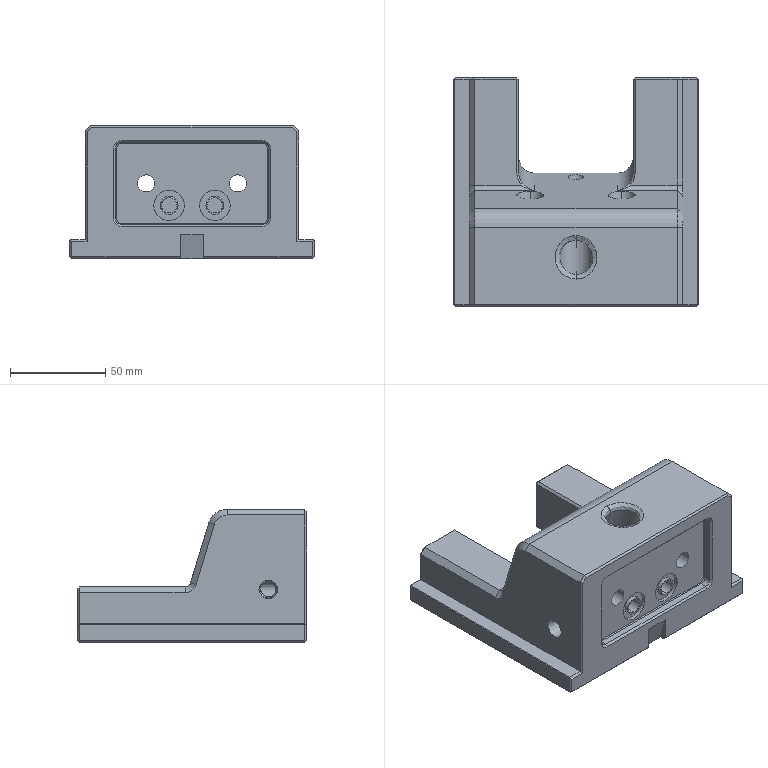Part | Creo | 1 solid | 225 faces | box 128 x 120 x 70 mm | volume 492923 mm3 | plane 108 | cylinder 73 | cone 28 | spline 12 | torus 4 | commonest cylinder face diameters 8 x26 6 x10 1.5 x8 16 x6 1 x4 9 x4